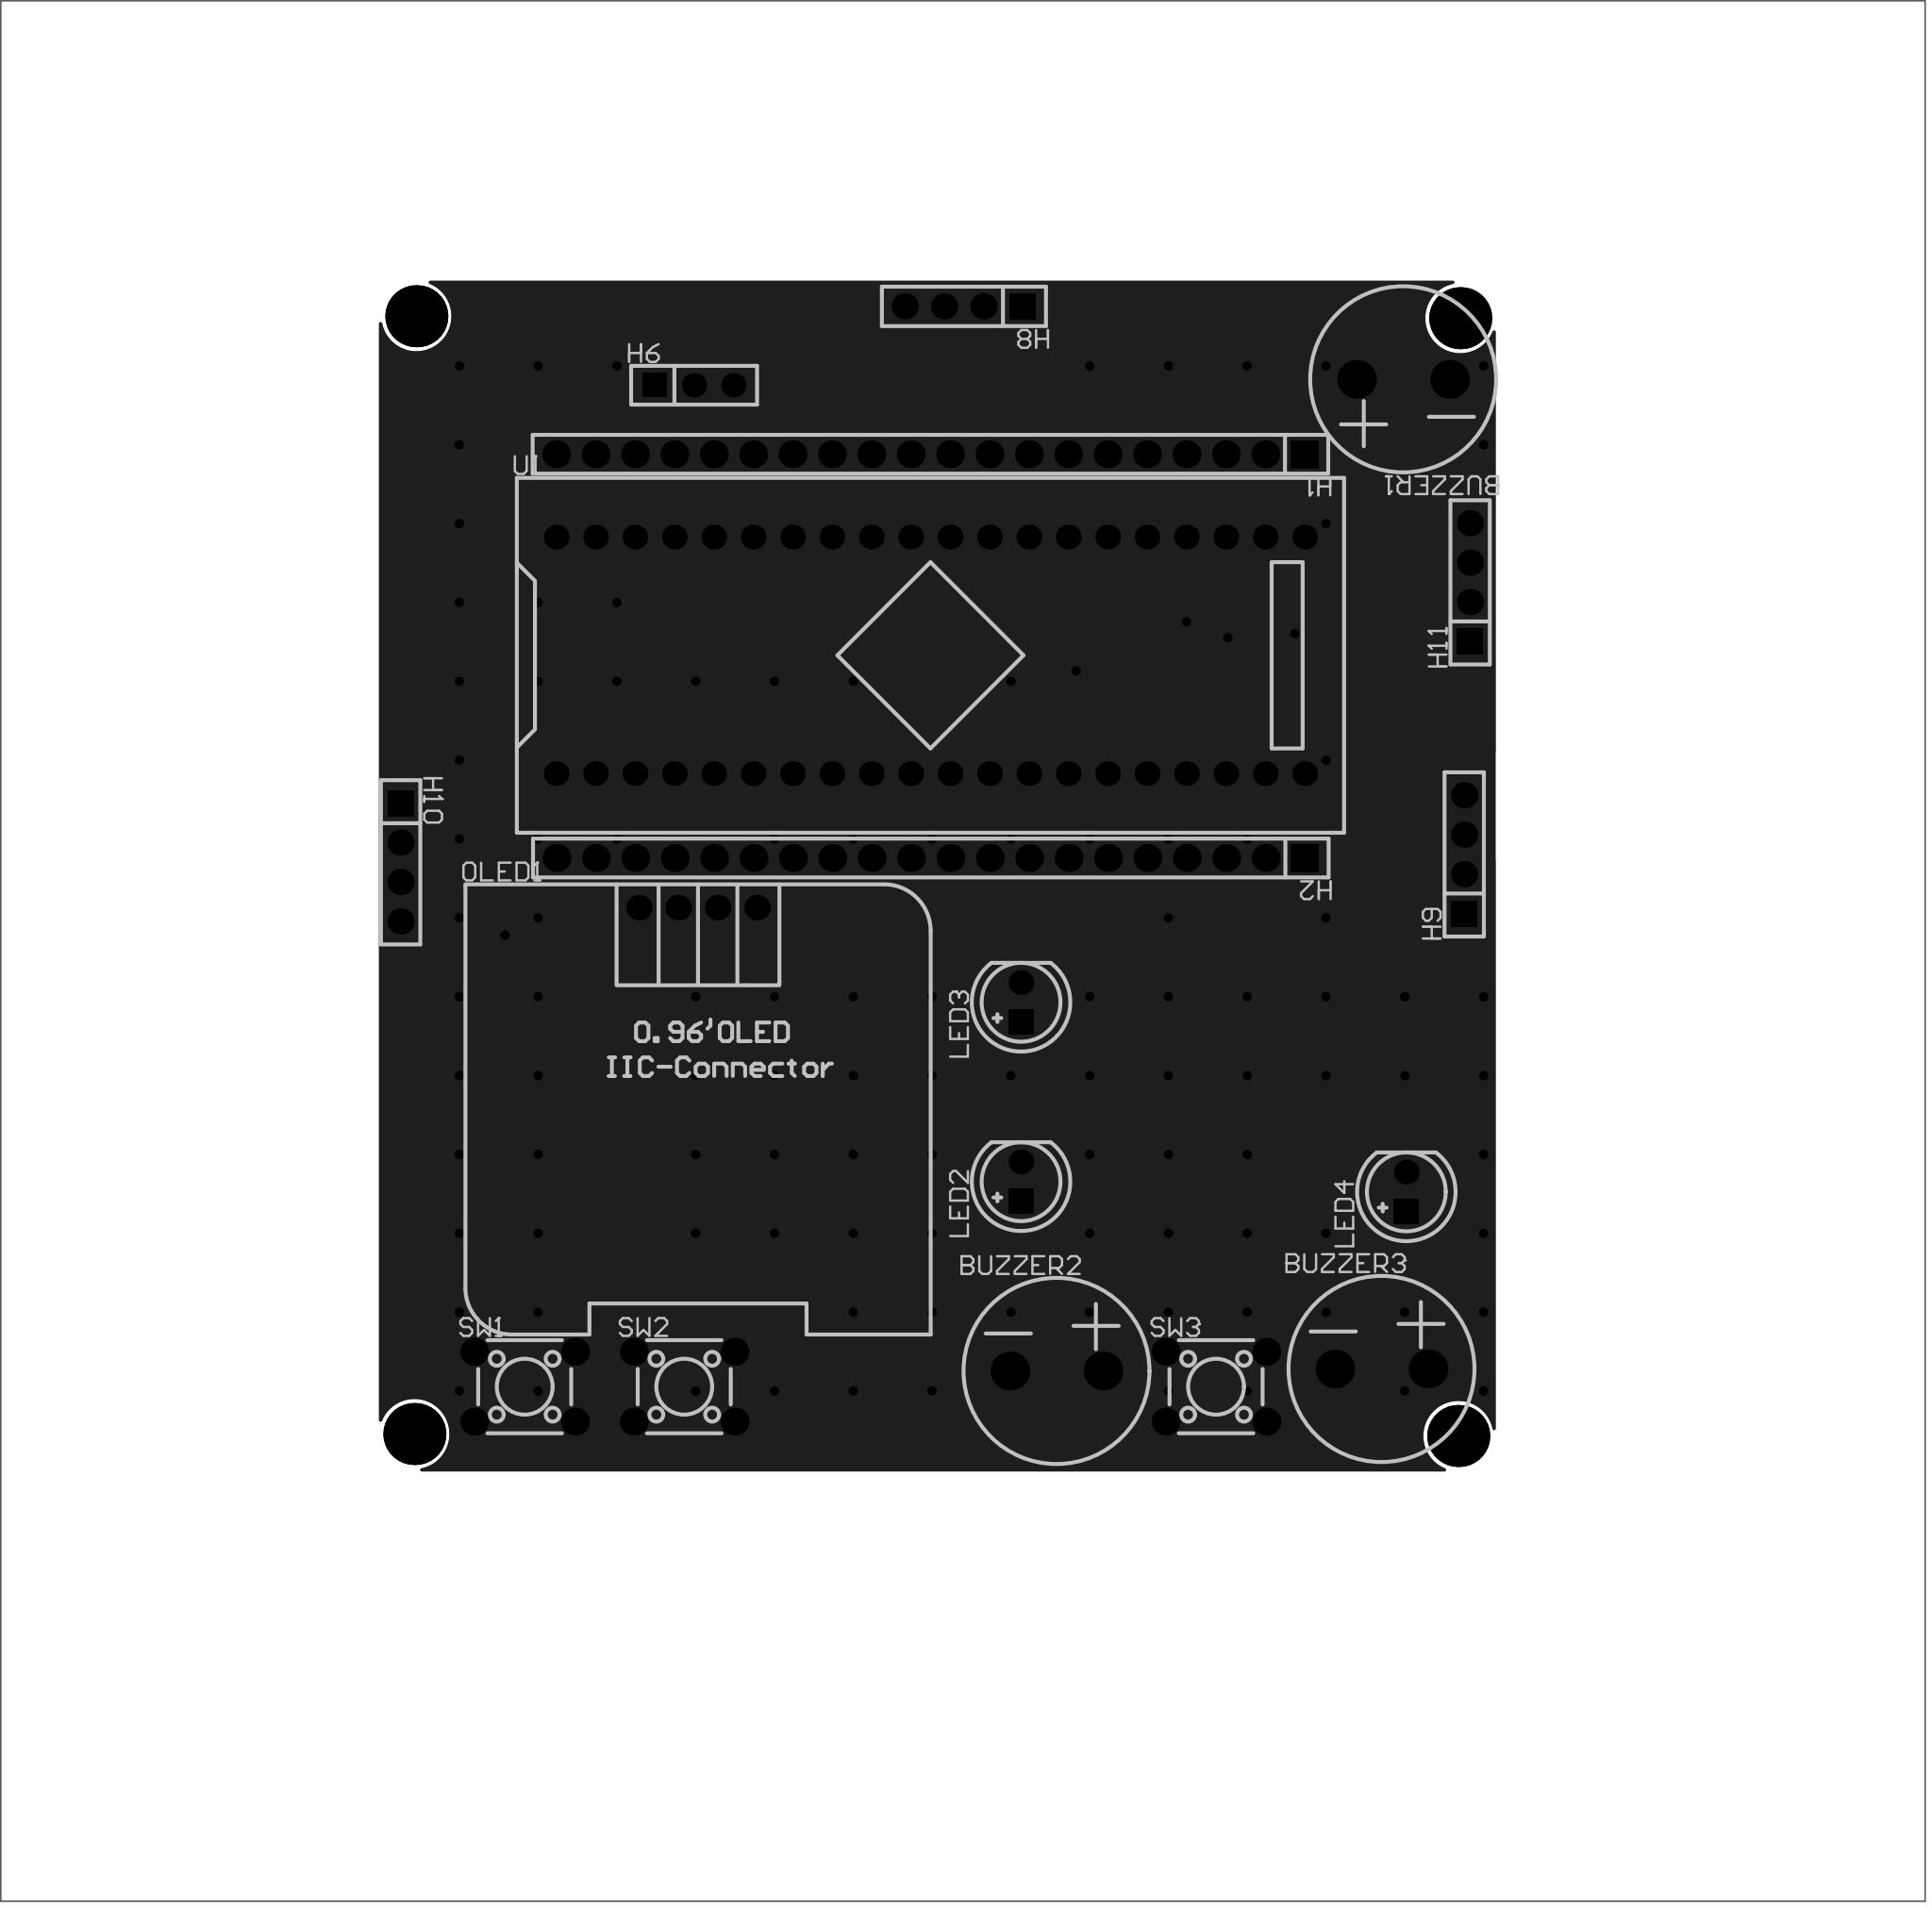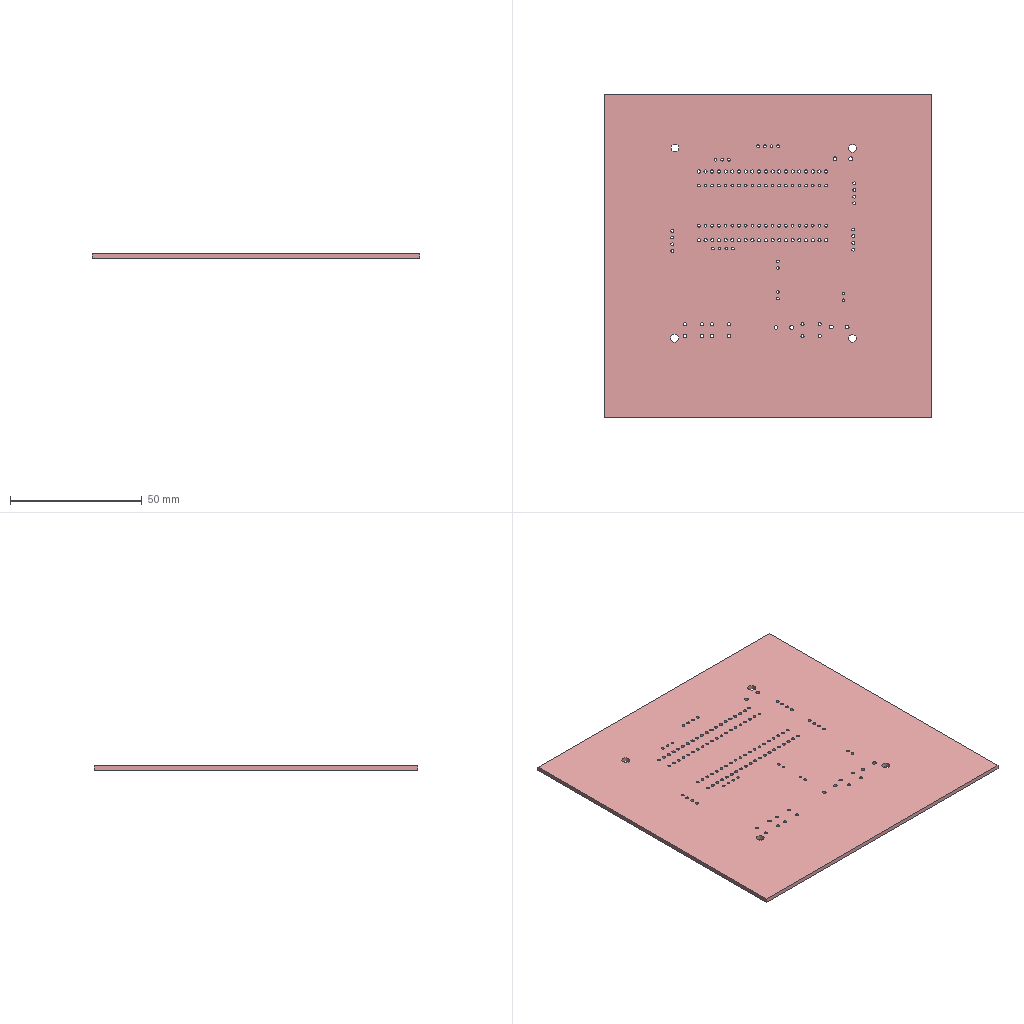Circuit board layout | Altium Designer | box 124.1 x 122.4 x 1.6 mm
Layer stack:
# Altium Designer layer stack of  (unit mm; dielectric type: 0 none, 1 core, 2 prepreg, 3 surface material)
index,name,kind,layer,copper_thickness_mm,dielectric_type,dielectric_thickness_mm,dielectric_material,dielectric_constant
0,Top Paste Mask Layer,other,,,,,,
1,Top Silkscreen Layer,other,,,,,,
2,Top Solder Mask Layer,dielectric,,,3,0.01,,3.3
3,Top Layer,copper,Top Layer,0.035,,,,
4,Dielectric1,dielectric,,,3,1.51,FR4,4.5
5,Bottom Layer,copper,Bottom Layer,0.035,,,,
6,Bottom Solder Mask Layer,dielectric,,,3,0.01,,3.3
7,Bottom Silkscreen Layer,other,,,,,,
8,Bottom Paste Mask Layer,other,,,,,,
# drill layer pairs: low layer,high layer
drill_pair,Top Layer,Bottom Layer
Part placement:
Designator,Comment,Layer,Footprint,Center-X(mm),Center-Y(mm),Rotation
BUZZER1,buzzer,TopLayer,BUZ-TH_BD12.0-P6.00-D0.9-RD,160.274,167.894,180
BUZZER2,buzzer,TopLayer,BUZ-TH_BD12.0-P6.00-D0.9-RD,137.922,104.013,0
BUZZER3,buzzer,TopLayer,BUZ-TH_BD12.0-P6.00-D0.9-RD,158.877,104.14,0
H1,,TopLayer,HDR-TH_20P-P2.54-V-F,129.794,163.068,180
H2,,TopLayer,HDR-TH_20P-P2.54-V-F,129.818,137.056,180
H6,,TopLayer,HDR-TH_3P-P2.54-V-F,114.554,167.513,0
H8,,TopLayer,HDR-TH_4P-P2.54-V-F,131.953,172.593,180
H9,,TopLayer,HDR-TH_4P-P2.54-V-F,164.211,137.287,90
H10,,TopLayer,HDR-TH_4P-P2.54-V-F,95.631,136.779,270
H11,,TopLayer,HDR-TH_4P-P2.54-V-F,164.592,154.813,90
LED2,,TopLayer,LED-TH_5mm,135.636,116.205,90
LED3,,TopLayer,LED-TH_5mm,135.636,127.762,90
LED4,,TopLayer,LED-TH_5mm,160.48,115.549,90
OLED1,,TopLayer,0.96OLED_4P,114.808,133.858,0
SW1,,TopLayer,SW-TH_4P-L6.0-W6.0-P4.50-LS6.5,103.632,102.997,0
SW2,,TopLayer,SW-TH_4P-L6.0-W6.0-P4.50-LS6.5,113.919,102.997,0
SW3,,TopLayer,SW-TH_4P-L6.0-W6.0-P4.50-LS6.5,148.209,102.997,0
U1,STM32F103C8T6-Card,TopLayer,CONN-TH_L53.3-W22.9_STM32F103C8T6-CARD,129.794,150.114,0
Pad and via stacks:
# Altium Designer via and pad stacks of  (unit mm). Each distinct definition once, with the count of objects using it.
# via: kind,start_layer,end_layer,hole_mm,diameter_mm,mode(0 simple;1 top-mid-bottom;2 full stack),diameter_per_layer,count,example_net
# pad: kind,layer,hole_mm,hole_type(0 round;1 square;2 slot),plating,top_size,top_shape(1 round;2 rect;3 octagon;9 rounded rect),mid_size,bottom_size,mode,footprint,size_per_layer,count,example
pad,Multi-Layer,3,0,plated,4x4,1,4x4,4x4,0,,,4,1
pad,Multi-Layer,1.5,0,plated,2.5x2.5,1,2.5x2.5,2.5x2.5,0,BUZ-TH_BD12.0-P6.00-D0.9-RD,,6,BUZZER1.1
pad,Multi-Layer,1.2,0,plated,1.8x1.8,2,1.8x1.8,1.8x1.8,0,HDR-TH_20P-P2.54-V-F,,2,H1.1
pad,Multi-Layer,1.2,0,plated,1.8x1.8,1,1.8x1.8,1.8x1.8,0,HDR-TH_20P-P2.54-V-F,,38,H1.2
pad,Multi-Layer,1.02,0,plated,1.575x1.575,1,1.575x1.575,1.575x1.575,0,HDR-TH_3P-P2.54-V-F,,2,H6.3
pad,Multi-Layer,1.02,0,plated,1.575x1.575,2,1.575x1.575,1.575x1.575,0,HDR-TH_3P-P2.54-V-F,,1,H6.1
pad,Multi-Layer,1.1,0,plated,1.7x1.7,2,1.7x1.7,1.7x1.7,0,HDR-TH_4P-P2.54-V-F,,4,H8.1
pad,Multi-Layer,1.1,0,plated,1.7x1.7,1,1.7x1.7,1.7x1.7,0,HDR-TH_4P-P2.54-V-F,,12,H8.2
pad,Multi-Layer,1,0,plated,1.6x1.6,2,1.6x1.6,1.6x1.6,0,LED-TH_5mm,,3,LED2.1
pad,Multi-Layer,1,0,plated,1.6x1.6,1,1.6x1.6,1.6x1.6,0,LED-TH_5mm,,3,LED2.2
pad,Multi-Layer,1,0,plated,1.65x1.65,1,1.65x1.65,1.65x1.65,0,0.96OLED_4P,,4,OLED1.4
pad,Multi-Layer,1.2,0,plated,1.8x1.8,1,1.8x1.8,1.8x1.8,0,SW-TH_4P-L6.0-W6.0-P4.50-LS6.5,,12,SW1.1
pad,Multi-Layer,1,0,plated,1.6x1.6,1,1.6x1.6,1.6x1.6,0,CONN-TH_L53.3-W22.9_STM32F103C8T6-CARD,,40,U1.1
via,Top Layer,Bottom Layer,0.3048,0.61,0,,110,PC14
Copper pours:
name,layer,net,type(0 solid;1 hatched;2 none)
Bottom Layer-GND,Bottom Layer,GND,0
Top Layer-GND,Top Layer,GND,0
Design rules, without the lines most boards share:
# Altium Designer design rules of  (exported by Altium Designer, unit mm)
# columns: name | kind | enabled | priority | scope1 | scope2 | descriptor | typed fields (field=value)
copperThickness1oz_2 | 2 | enabled | 2 | All | All | Width Constraint (Min=5mil) (Max=100mil) (Preferred=30mil) (All) |
viaSize | 11 | enabled | 1 | All | All | Routing Via (MinHoleWidth=11.811mil) (MaxHoleWidth=248.032mil) (PreferredHoleWidth=12.008mil) (MinWidth=19.685mil) (MaxWidth=393.701mil) (PreferedWidth=24.016mil) (All) | via_min_hole=0.3 via_max_hole=6.3 via_preferred_diameter=0.61 via_preferred_hole=0.305
solderMaskExpansion | 13 | enabled | 2 | All | All | Solder Mask Expansion (Expansion =2.008mil) (All) | expansion=0.051